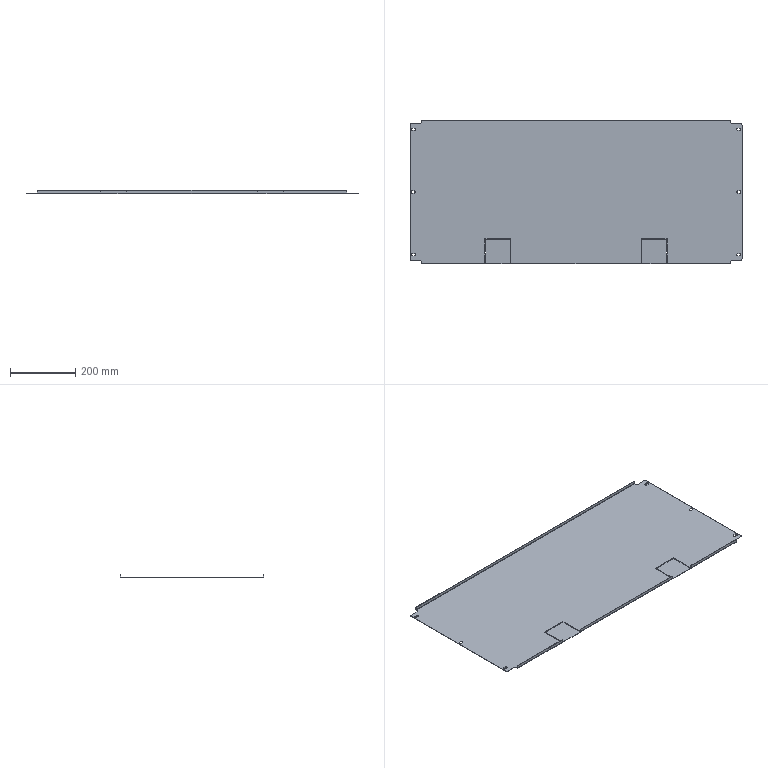Part | SolidWorks | features ICE 4, SMBaseFlange 2, Cut 1, EdgeFlange 1, Fillet 1, FlatPattern 1, SheetMetal 1 | 1 solid | 124 faces | box 1020 x 441 x 10 mm | volume 461945 mm3 | plane 90 | cylinder 34 | commonest cylinder face diameters 7 x18 10 x8 1 x4 3 x4